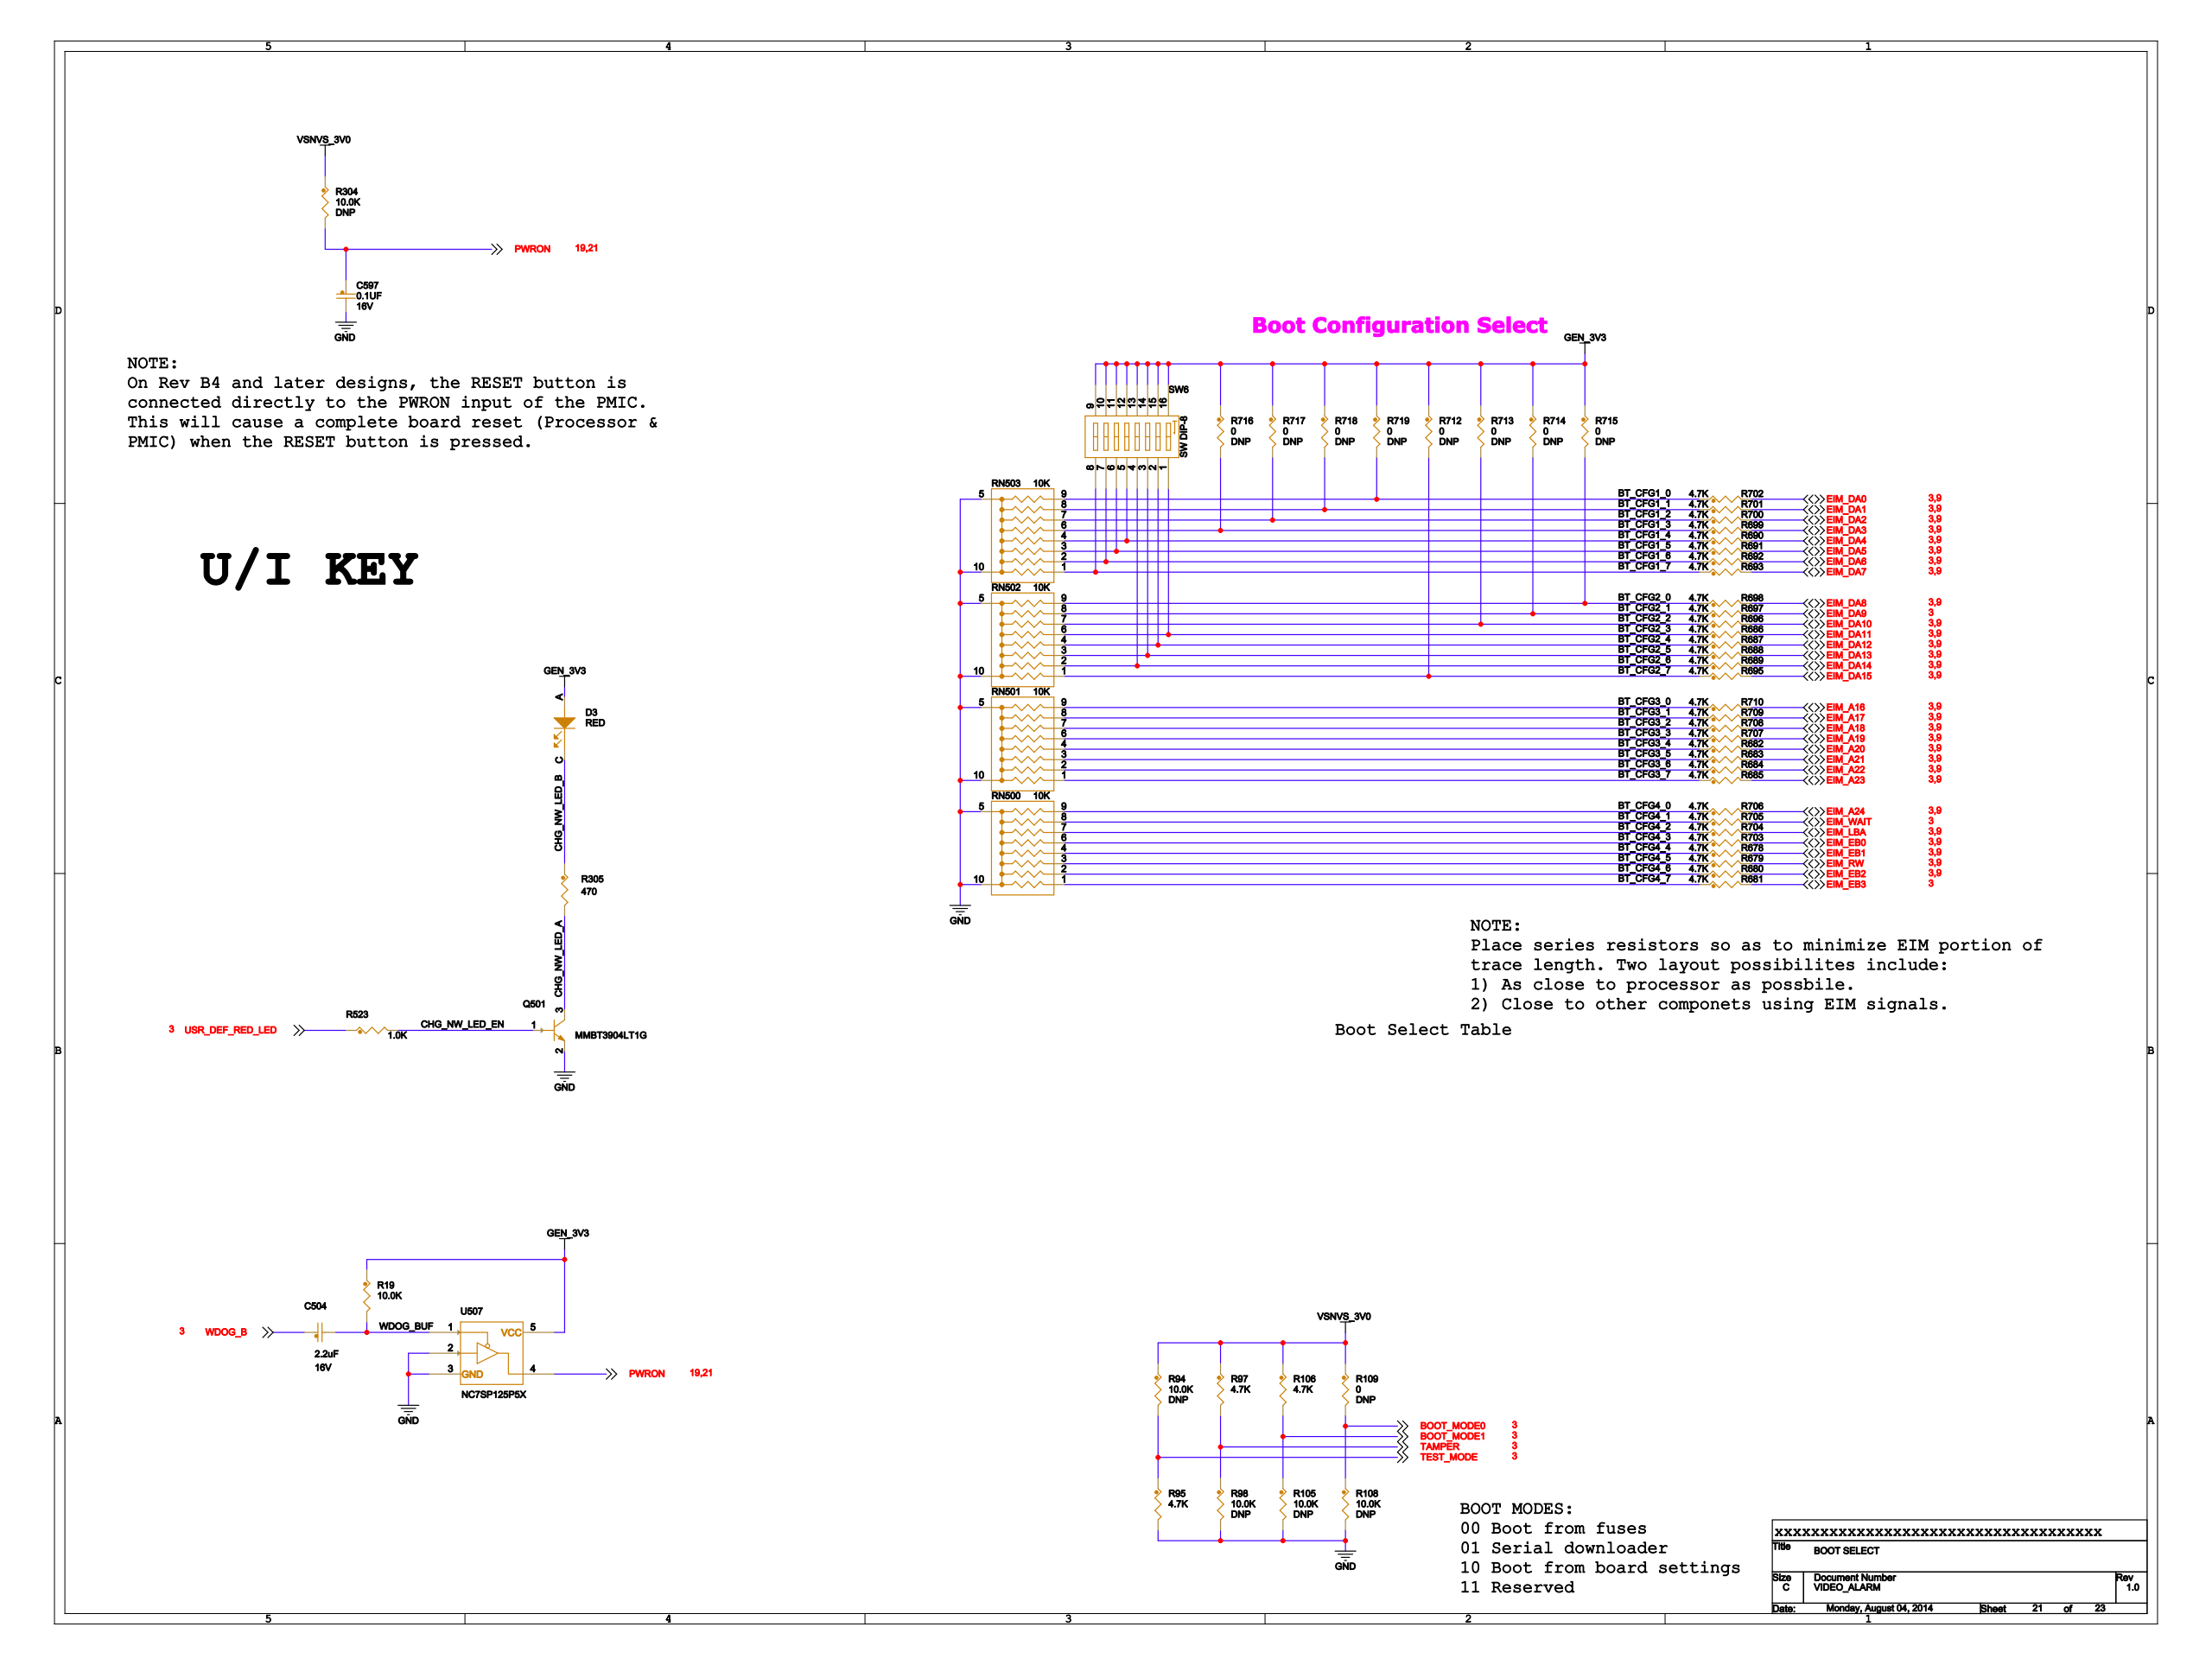Circuit board | Cadence Allegro | 994 parts | 728 nets | one sheet of the schematic
Parts on this sheet (reference | value | footprint):
C504 | 2.2uF | 0603_CC
C597 | 0.1UF | 0402_CC
D3 | RED | LED_0603
Q501 | MMBT3904LT1G | SOT23
R19 | 10.0K | 0603_CC
R94 | 10.0K | 0603_CC
R95 | 4.7K | 0603_CC
R97 | 4.7K | 0603_CC
R98 | 10.0K | 0603_CC
R105 | 10.0K | 0603_CC
R106 | 4.7K | 0603_CC
R108 | 10.0K | 0603_CC
R109 | 0 | 0603_CC
R304 | 10.0K | 0402_CC
R305 | 470 | 0603_CC
R523 | 1.0K | 0603_CC
R678 | 4.7K | 0402_CC
R679 | 4.7K | 0402_CC
R680 | 4.7K | 0402_CC
R681 | 4.7K | 0402_CC
R682 | 4.7K | 0402_CC
R683 | 4.7K | 0402_CC
R684 | 4.7K | 0402_CC
R685 | 4.7K | 0402_CC
R686 | 4.7K | 0402_CC
R687 | 4.7K | 0402_CC
R688 | 4.7K | 0402_CC
R689 | 4.7K | 0402_CC
R690 | 4.7K | 0402_CC
R691 | 4.7K | 0402_CC
R692 | 4.7K | 0402_CC
R693 | 4.7K | 0402_CC
R695 | 4.7K | 0402_CC
R696 | 4.7K | 0402_CC
R697 | 4.7K | 0402_CC
R698 | 4.7K | 0402_CC
R699 | 4.7K | 0402_CC
R700 | 4.7K | 0402_CC
R701 | 4.7K | 0402_CC
R702 | 4.7K | 0402_CC
R703 | 4.7K | 0402_CC
R704 | 4.7K | 0402_CC
R705 | 4.7K | 0402_CC
R706 | 4.7K | 0402_CC
R707 | 4.7K | 0402_CC
R708 | 4.7K | 0402_CC
R709 | 4.7K | 0402_CC
R710 | 4.7K | 0402_CC
R712 | 0 | 0603_CC
R713 | 0 | 0603_CC
R714 | 0 | 0603_CC
R715 | 0 | 0603_CC
R716 | 0 | 0603_CC
R717 | 0 | 0603_CC
R718 | 0 | 0603_CC
R719 | 0 | 0603_CC
RN500 | 10K | RCA_8_10
RN501 | 10K | RCA_8_10
RN502 | 10K | RCA_8_10
RN503 | 10K | RCA_8_10
U507 | NC7SP125P5X | SC70-5_A
Nets of these parts (net: part-pin ...):
GND: C597-2 Q501-2 R95-2 R98-2 R105-2 R108-2 RN500-5 RN500-10 RN501-5 RN501-10 RN502-5 RN502-10 RN503-5 RN503-10 U507-2 U507-3
PWRON: C597-1 R304-2 U507-4
GEN_3V3: D3-A R19-1 R712-1 R713-1 R714-1 R715-1 R716-1 R717-1 R718-1 R719-1 U507-5
BT_CFG1_0: R702-1 R719-2 RN503-9
BT_CFG1_1: R701-1 R718-2 RN503-8
BT_CFG1_2: R700-1 R717-2 RN503-7
BT_CFG1_3: R699-1 R716-2 RN503-6
BT_CFG2_0: R698-1 R715-2 RN502-9
BT_CFG2_1: R697-1 R714-2 RN502-8
BT_CFG2_2: R696-1 R713-2 RN502-7
BT_CFG2_7: R695-1 R712-2 RN502-1
VSNVS_3V0: R94-1 R97-1 R106-1 R109-1 R304-1
BOOT_MODE0: R108-1 R109-2
TAMPER: R97-2 R98-1
TEST_MODE: R94-2 R95-1
WDOG_BUF: C504-2 R19-2 U507-1
BOOT_MODE1: R105-1 R106-2
EIM_A16: R710-2
EIM_A17: R709-2
EIM_A18: R708-2
EIM_A19: R707-2
EIM_A20: R682-2
EIM_A21: R683-2
EIM_A22: R684-2
EIM_A23: R685-2
EIM_A24: R706-2
EIM_DA0: R702-2
EIM_DA1: R701-2
EIM_DA10: R696-2
EIM_DA11: R686-2
EIM_DA12: R687-2
EIM_DA13: R688-2
EIM_DA14: R689-2
EIM_DA15: R695-2
EIM_DA2: R700-2
EIM_DA3: R699-2
EIM_DA4: R690-2
EIM_DA5: R691-2
EIM_DA6: R692-2
EIM_DA7: R693-2
EIM_DA8: R698-2
EIM_DA9: R697-2
EIM_EB0: R703-2
EIM_EB1: R678-2
EIM_EB2: R680-2
EIM_EB3: R681-2
EIM_LBA: R704-2
EIM_RW: R679-2
EIM_WAIT: R705-2
BT_CFG2_3: R686-1 RN502-6
BT_CFG2_4: R687-1 RN502-4
BT_CFG2_5: R688-1 RN502-3
BT_CFG2_6: R689-1 RN502-2
BT_CFG1_4: R690-1 RN503-4
BT_CFG1_5: R691-1 RN503-3
BT_CFG1_6: R692-1 RN503-2
BT_CFG1_7: R693-1 RN503-1
BT_CFG3_7: R685-1 RN501-1
BT_CFG3_6: R684-1 RN501-2
BT_CFG3_5: R683-1 RN501-3
BT_CFG3_4: R682-1 RN501-4
BT_CFG3_3: R707-1 RN501-6
BT_CFG3_2: R708-1 RN501-7
BT_CFG3_1: R709-1 RN501-8
BT_CFG3_0: R710-1 RN501-9
BT_CFG4_7: R681-1 RN500-1
BT_CFG4_6: R680-1 RN500-2
BT_CFG4_5: R679-1 RN500-3
BT_CFG4_4: R678-1 RN500-4
BT_CFG4_3: R703-1 RN500-6
BT_CFG4_2: R704-1 RN500-7
BT_CFG4_1: R705-1 RN500-8
BT_CFG4_0: R706-1 RN500-9
USR_DEF_RED_LED: R523-1
CHG_NW_LED_EN: Q501-1 R523-2
CHG_NW_LED_B: D3-C R305-1
CHG_NW_LED_A: Q501-3 R305-2
WDOG_B: C504-1